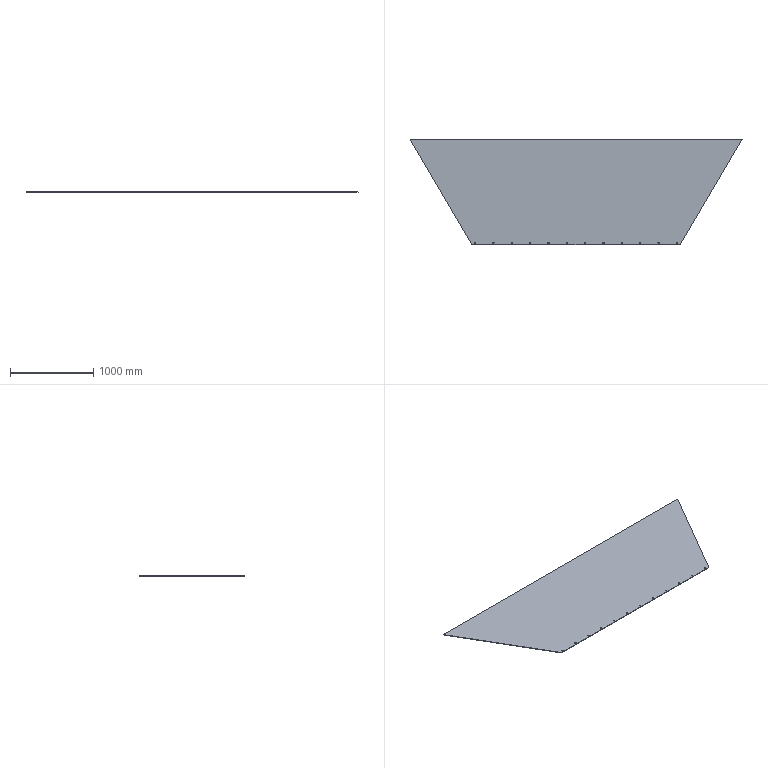Part | SolidWorks | features ICE 3, LPattern 2, FlatPattern 1, SMBaseFlange 1, SheetMetal 1 | 1 solid | 30 faces | box 3983 x 1270 x 6 mm | volume 24689146 mm3 | cylinder 24 | plane 6 | commonest cylinder face diameters 14 x24
STEP:
#1=CARTESIAN_POINT('',(-1203.,-610.,-6.));
#2=VERTEX_POINT('',#1);
#3=CARTESIAN_POINT('',(-1217.,-610.,-6.));
#4=VERTEX_POINT('',#3);
#5=CARTESIAN_POINT('',(-1210.,-610.,-6.));
#6=DIRECTION('',(0.,0.,-1.));
#7=DIRECTION('',(1.,0.,0.));
#8=AXIS2_PLACEMENT_3D('',#5,#6,#7);
#9=CIRCLE('',#8,7.);
#10=EDGE_CURVE('',#2,#4,#9,.T.);
#11=ORIENTED_EDGE('',*,*,#10,.T.);
#12=CARTESIAN_POINT('',(-1217.,-610.,0.));
#13=VERTEX_POINT('',#12);
#14=CARTESIAN_POINT('',(-1217.,-610.,-6.001));
#15=DIRECTION('',(0.,0.,1.));
#16=VECTOR('',#15,1000.);
#17=LINE('',#14,#16);
#18=EDGE_CURVE('',#4,#13,#17,.T.);
#19=ORIENTED_EDGE('',*,*,#18,.T.);
#20=CARTESIAN_POINT('',(-1203.,-610.,0.));
#21=VERTEX_POINT('',#20);
#22=CARTESIAN_POINT('',(-1210.,-610.,0.));
#23=DIRECTION('',(0.,0.,1.));
#24=DIRECTION('',(1.,0.,0.));
#25=AXIS2_PLACEMENT_3D('',#22,#23,#24);
#26=CIRCLE('',#25,7.);
#27=EDGE_CURVE('',#13,#21,#26,.T.);
#28=ORIENTED_EDGE('',*,*,#27,.T.);
#29=CARTESIAN_POINT('',(-1203.,-610.,-6.001));
#30=DIRECTION('',(0.,0.,1.));
#31=VECTOR('',#30,1000.);
#32=LINE('',#29,#31);
#33=EDGE_CURVE('',#2,#21,#32,.T.);
#34=ORIENTED_EDGE('',*,*,#33,.F.);
#35=EDGE_LOOP('',(#11,#19,#28,#34));
#36=FACE_OUTER_BOUND('',#35,.T.);
#37=CARTESIAN_POINT('',(-1210.,-610.,-6.001));
#38=DIRECTION('',(0.,0.,1.));
#39=DIRECTION('',(1.,0.,0.));
#40=AXIS2_PLACEMENT_3D('',#37,#38,#39);
#41=CYLINDRICAL_SURFACE('',#40,7.);
#42=ADVANCED_FACE('',(#36),#41,.F.);
#43=CARTESIAN_POINT('',(-983.,-610.,-6.));
#44=VERTEX_POINT('',#43);
#45=CARTESIAN_POINT('',(-997.,-610.,-6.));
#46=VERTEX_POINT('',#45);
#47=CARTESIAN_POINT('',(-990.,-610.,-6.));
#48=DIRECTION('',(0.,0.,-1.));
#49=DIRECTION('',(1.,0.,0.));
#50=AXIS2_PLACEMENT_3D('',#47,#48,#49);
#51=CIRCLE('',#50,7.);
#52=EDGE_CURVE('',#44,#46,#51,.T.);
#53=ORIENTED_EDGE('',*,*,#52,.T.);
#54=CARTESIAN_POINT('',(-997.,-610.,0.));
#55=VERTEX_POINT('',#54);
#56=CARTESIAN_POINT('',(-997.,-610.,-6.001));
#57=DIRECTION('',(0.,0.,1.));
#58=VECTOR('',#57,1000.);
#59=LINE('',#56,#58);
#60=EDGE_CURVE('',#46,#55,#59,.T.);
#61=ORIENTED_EDGE('',*,*,#60,.T.);
#62=CARTESIAN_POINT('',(-983.,-610.,0.));
#63=VERTEX_POINT('',#62);
#64=CARTESIAN_POINT('',(-990.,-610.,0.));
#65=DIRECTION('',(0.,0.,1.));
#66=DIRECTION('',(1.,0.,0.));
#67=AXIS2_PLACEMENT_3D('',#64,#65,#66);
#68=CIRCLE('',#67,7.);
#69=EDGE_CURVE('',#55,#63,#68,.T.);
#70=ORIENTED_EDGE('',*,*,#69,.T.);
#71=CARTESIAN_POINT('',(-983.,-610.,-6.001));
#72=DIRECTION('',(0.,0.,1.));
#73=VECTOR('',#72,1000.);
#74=LINE('',#71,#73);
#75=EDGE_CURVE('',#44,#63,#74,.T.);
#76=ORIENTED_EDGE('',*,*,#75,.F.);
#77=EDGE_LOOP('',(#53,#61,#70,#76));
#78=FACE_OUTER_BOUND('',#77,.T.);
#79=CARTESIAN_POINT('',(-990.,-610.,-6.001));
#80=DIRECTION('',(0.,0.,1.));
#81=DIRECTION('',(1.,0.,0.));
#82=AXIS2_PLACEMENT_3D('',#79,#80,#81);
#83=CYLINDRICAL_SURFACE('',#82,7.);
#84=ADVANCED_FACE('',(#78),#83,.F.);
#85=CARTESIAN_POINT('',(-763.,-610.,-6.));
#86=VERTEX_POINT('',#85);
#87=CARTESIAN_POINT('',(-777.,-610.,-6.));
#88=VERTEX_POINT('',#87);
#89=CARTESIAN_POINT('',(-770.,-610.,-6.));
#90=DIRECTION('',(0.,0.,-1.));
#91=DIRECTION('',(1.,0.,0.));
#92=AXIS2_PLACEMENT_3D('',#89,#90,#91);
#93=CIRCLE('',#92,7.);
#94=EDGE_CURVE('',#86,#88,#93,.T.);
#95=ORIENTED_EDGE('',*,*,#94,.T.);
#96=CARTESIAN_POINT('',(-777.,-610.,0.));
#97=VERTEX_POINT('',#96);
#98=CARTESIAN_POINT('',(-777.,-610.,-6.001));
#99=DIRECTION('',(0.,0.,1.));
#100=VECTOR('',#99,1000.);
#101=LINE('',#98,#100);
#102=EDGE_CURVE('',#88,#97,#101,.T.);
#103=ORIENTED_EDGE('',*,*,#102,.T.);
#104=CARTESIAN_POINT('',(-763.,-610.,0.));
#105=VERTEX_POINT('',#104);
#106=CARTESIAN_POINT('',(-770.,-610.,0.));
#107=DIRECTION('',(0.,0.,1.));
#108=DIRECTION('',(1.,0.,0.));
#109=AXIS2_PLACEMENT_3D('',#106,#107,#108);
#110=CIRCLE('',#109,7.);
#111=EDGE_CURVE('',#97,#105,#110,.T.);
#112=ORIENTED_EDGE('',*,*,#111,.T.);
#113=CARTESIAN_POINT('',(-763.,-610.,-6.001));
#114=DIRECTION('',(0.,0.,1.));
#115=VECTOR('',#114,1000.);
#116=LINE('',#113,#115);
#117=EDGE_CURVE('',#86,#105,#116,.T.);
#118=ORIENTED_EDGE('',*,*,#117,.F.);
#119=EDGE_LOOP('',(#95,#103,#112,#118));
#120=FACE_OUTER_BOUND('',#119,.T.);
#121=CARTESIAN_POINT('',(-770.,-610.,-6.001));
#122=DIRECTION('',(0.,0.,1.));
#123=DIRECTION('',(1.,0.,0.));
#124=AXIS2_PLACEMENT_3D('',#121,#122,#123);
#125=CYLINDRICAL_SURFACE('',#124,7.);
#126=ADVANCED_FACE('',(#120),#125,.F.);
#127=CARTESIAN_POINT('',(-543.,-610.,-6.));
#128=VERTEX_POINT('',#127);
#129=CARTESIAN_POINT('',(-557.,-610.,-6.));
#130=VERTEX_POINT('',#129);
#131=CARTESIAN_POINT('',(-550.,-610.,-6.));
#132=DIRECTION('',(0.,0.,-1.));
#133=DIRECTION('',(1.,0.,0.));
#134=AXIS2_PLACEMENT_3D('',#131,#132,#133);
#135=CIRCLE('',#134,7.);
#136=EDGE_CURVE('',#128,#130,#135,.T.);
#137=ORIENTED_EDGE('',*,*,#136,.T.);
#138=CARTESIAN_POINT('',(-557.,-610.,0.));
#139=VERTEX_POINT('',#138);
#140=CARTESIAN_POINT('',(-557.,-610.,-6.001));
#141=DIRECTION('',(0.,0.,1.));
#142=VECTOR('',#141,1000.);
#143=LINE('',#140,#142);
#144=EDGE_CURVE('',#130,#139,#143,.T.);
#145=ORIENTED_EDGE('',*,*,#144,.T.);
#146=CARTESIAN_POINT('',(-543.,-610.,0.));
#147=VERTEX_POINT('',#146);
#148=CARTESIAN_POINT('',(-550.,-610.,0.));
#149=DIRECTION('',(0.,0.,1.));
#150=DIRECTION('',(1.,0.,0.));
#151=AXIS2_PLACEMENT_3D('',#148,#149,#150);
#152=CIRCLE('',#151,7.);
#153=EDGE_CURVE('',#139,#147,#152,.T.);
#154=ORIENTED_EDGE('',*,*,#153,.T.);
#155=CARTESIAN_POINT('',(-543.,-610.,-6.001));
#156=DIRECTION('',(0.,0.,1.));
#157=VECTOR('',#156,1000.);
#158=LINE('',#155,#157);
#159=EDGE_CURVE('',#128,#147,#158,.T.);
#160=ORIENTED_EDGE('',*,*,#159,.F.);
#161=EDGE_LOOP('',(#137,#145,#154,#160));
#162=FACE_OUTER_BOUND('',#161,.T.);
#163=CARTESIAN_POINT('',(-550.,-610.,-6.001));
#164=DIRECTION('',(0.,0.,1.));
#165=DIRECTION('',(1.,0.,0.));
#166=AXIS2_PLACEMENT_3D('',#163,#164,#165);
#167=CYLINDRICAL_SURFACE('',#166,7.);
#168=ADVANCED_FACE('',(#162),#167,.F.);
#169=CARTESIAN_POINT('',(-323.,-610.,-6.));
#170=VERTEX_POINT('',#169);
#171=CARTESIAN_POINT('',(-337.,-610.,-6.));
#172=VERTEX_POINT('',#171);
#173=CARTESIAN_POINT('',(-330.,-610.,-6.));
#174=DIRECTION('',(0.,0.,-1.));
#175=DIRECTION('',(1.,0.,0.));
#176=AXIS2_PLACEMENT_3D('',#173,#174,#175);
#177=CIRCLE('',#176,7.);
#178=EDGE_CURVE('',#170,#172,#177,.T.);
#179=ORIENTED_EDGE('',*,*,#178,.T.);
#180=CARTESIAN_POINT('',(-337.,-610.,0.));
#181=VERTEX_POINT('',#180);
#182=CARTESIAN_POINT('',(-337.,-610.,-6.001));
#183=DIRECTION('',(0.,0.,1.));
#184=VECTOR('',#183,1000.);
#185=LINE('',#182,#184);
#186=EDGE_CURVE('',#172,#181,#185,.T.);
#187=ORIENTED_EDGE('',*,*,#186,.T.);
#188=CARTESIAN_POINT('',(-323.,-610.,0.));
#189=VERTEX_POINT('',#188);
#190=CARTESIAN_POINT('',(-330.,-610.,0.));
#191=DIRECTION('',(0.,0.,1.));
#192=DIRECTION('',(1.,0.,0.));
#193=AXIS2_PLACEMENT_3D('',#190,#191,#192);
#194=CIRCLE('',#193,7.);
#195=EDGE_CURVE('',#181,#189,#194,.T.);
#196=ORIENTED_EDGE('',*,*,#195,.T.);
#197=CARTESIAN_POINT('',(-323.,-610.,-6.001));
#198=DIRECTION('',(0.,0.,1.));
#199=VECTOR('',#198,1000.);
#200=LINE('',#197,#199);
#201=EDGE_CURVE('',#170,#189,#200,.T.);
#202=ORIENTED_EDGE('',*,*,#201,.F.);
#203=EDGE_LOOP('',(#179,#187,#196,#202));
#204=FACE_OUTER_BOUND('',#203,.T.);
#205=CARTESIAN_POINT('',(-330.,-610.,-6.001));
#206=DIRECTION('',(0.,0.,1.));
#207=DIRECTION('',(1.,0.,0.));
#208=AXIS2_PLACEMENT_3D('',#205,#206,#207);
#209=CYLINDRICAL_SURFACE('',#208,7.);
#210=ADVANCED_FACE('',(#204),#209,.F.);
#211=CARTESIAN_POINT('',(1203.,-610.,-6.));
#212=VERTEX_POINT('',#211);
#213=CARTESIAN_POINT('',(1217.,-610.,-6.));
#214=VERTEX_POINT('',#213);
#215=CARTESIAN_POINT('',(1210.,-610.,-6.));
#216=DIRECTION('',(0.,0.,1.));
#217=DIRECTION('',(1.,0.,0.));
#218=AXIS2_PLACEMENT_3D('',#215,#216,#217);
#219=CIRCLE('',#218,7.);
#220=EDGE_CURVE('',#212,#214,#219,.T.);
#221=ORIENTED_EDGE('',*,*,#220,.F.);
#222=CARTESIAN_POINT('',(1203.,-610.,0.));
#223=VERTEX_POINT('',#222);
#224=CARTESIAN_POINT('',(1203.,-610.,-10.));
#225=DIRECTION('',(0.,0.,1.));
#226=VECTOR('',#225,1000.);
#227=LINE('',#224,#226);
#228=EDGE_CURVE('',#212,#223,#227,.T.);
#229=ORIENTED_EDGE('',*,*,#228,.T.);
#230=CARTESIAN_POINT('',(1217.,-610.,0.));
#231=VERTEX_POINT('',#230);
#232=CARTESIAN_POINT('',(1210.,-610.,0.));
#233=DIRECTION('',(0.,0.,1.));
#234=DIRECTION('',(1.,0.,0.));
#235=AXIS2_PLACEMENT_3D('',#232,#233,#234);
#236=CIRCLE('',#235,7.);
#237=EDGE_CURVE('',#223,#231,#236,.T.);
#238=ORIENTED_EDGE('',*,*,#237,.T.);
#239=CARTESIAN_POINT('',(1217.,-610.,-10.));
#240=DIRECTION('',(0.,0.,1.));
#241=VECTOR('',#240,1000.);
#242=LINE('',#239,#241);
#243=EDGE_CURVE('',#214,#231,#242,.T.);
#244=ORIENTED_EDGE('',*,*,#243,.F.);
#245=EDGE_LOOP('',(#221,#229,#238,#244));
#246=FACE_OUTER_BOUND('',#245,.T.);
#247=CARTESIAN_POINT('',(1210.,-610.,-10.));
#248=DIRECTION('',(0.,0.,1.));
#249=DIRECTION('',(1.,0.,0.));
#250=AXIS2_PLACEMENT_3D('',#247,#248,#249);
#251=CYLINDRICAL_SURFACE('',#250,7.);
#252=ADVANCED_FACE('',(#246),#251,.F.);
#253=CARTESIAN_POINT('',(983.,-610.,-6.));
#254=VERTEX_POINT('',#253);
#255=CARTESIAN_POINT('',(997.,-610.,-6.));
#256=VERTEX_POINT('',#255);
#257=CARTESIAN_POINT('',(990.,-610.,-6.));
#258=DIRECTION('',(0.,0.,1.));
#259=DIRECTION('',(1.,0.,0.));
#260=AXIS2_PLACEMENT_3D('',#257,#258,#259);
#261=CIRCLE('',#260,7.);
#262=EDGE_CURVE('',#254,#256,#261,.T.);
#263=ORIENTED_EDGE('',*,*,#262,.F.);
#264=CARTESIAN_POINT('',(983.,-610.,0.));
#265=VERTEX_POINT('',#264);
#266=CARTESIAN_POINT('',(983.,-610.,-10.));
#267=DIRECTION('',(0.,0.,1.));
#268=VECTOR('',#267,1000.);
#269=LINE('',#266,#268);
#270=EDGE_CURVE('',#254,#265,#269,.T.);
#271=ORIENTED_EDGE('',*,*,#270,.T.);
#272=CARTESIAN_POINT('',(997.,-610.,0.));
#273=VERTEX_POINT('',#272);
#274=CARTESIAN_POINT('',(990.,-610.,0.));
#275=DIRECTION('',(0.,0.,1.));
#276=DIRECTION('',(1.,0.,0.));
#277=AXIS2_PLACEMENT_3D('',#274,#275,#276);
#278=CIRCLE('',#277,7.);
#279=EDGE_CURVE('',#265,#273,#278,.T.);
#280=ORIENTED_EDGE('',*,*,#279,.T.);
#281=CARTESIAN_POINT('',(997.,-610.,-10.));
#282=DIRECTION('',(0.,0.,1.));
#283=VECTOR('',#282,1000.);
#284=LINE('',#281,#283);
#285=EDGE_CURVE('',#256,#273,#284,.T.);
#286=ORIENTED_EDGE('',*,*,#285,.F.);
#287=EDGE_LOOP('',(#263,#271,#280,#286));
#288=FACE_OUTER_BOUND('',#287,.T.);
#289=CARTESIAN_POINT('',(990.,-610.,-10.));
#290=DIRECTION('',(0.,0.,1.));
#291=DIRECTION('',(1.,0.,0.));
#292=AXIS2_PLACEMENT_3D('',#289,#290,#291);
#293=CYLINDRICAL_SURFACE('',#292,7.);
#294=ADVANCED_FACE('',(#288),#293,.F.);
#295=CARTESIAN_POINT('',(763.,-610.,-6.));
#296=VERTEX_POINT('',#295);
#297=CARTESIAN_POINT('',(777.,-610.,-6.));
#298=VERTEX_POINT('',#297);
#299=CARTESIAN_POINT('',(770.,-610.,-6.));
#300=DIRECTION('',(0.,0.,1.));
#301=DIRECTION('',(1.,0.,0.));
#302=AXIS2_PLACEMENT_3D('',#299,#300,#301);
#303=CIRCLE('',#302,7.);
#304=EDGE_CURVE('',#296,#298,#303,.T.);
#305=ORIENTED_EDGE('',*,*,#304,.F.);
#306=CARTESIAN_POINT('',(763.,-610.,0.));
#307=VERTEX_POINT('',#306);
#308=CARTESIAN_POINT('',(763.,-610.,-10.));
#309=DIRECTION('',(0.,0.,1.));
#310=VECTOR('',#309,1000.);
#311=LINE('',#308,#310);
#312=EDGE_CURVE('',#296,#307,#311,.T.);
#313=ORIENTED_EDGE('',*,*,#312,.T.);
#314=CARTESIAN_POINT('',(777.,-610.,0.));
#315=VERTEX_POINT('',#314);
#316=CARTESIAN_POINT('',(770.,-610.,0.));
#317=DIRECTION('',(0.,0.,1.));
#318=DIRECTION('',(1.,0.,0.));
#319=AXIS2_PLACEMENT_3D('',#316,#317,#318);
#320=CIRCLE('',#319,7.);
#321=EDGE_CURVE('',#307,#315,#320,.T.);
#322=ORIENTED_EDGE('',*,*,#321,.T.);
#323=CARTESIAN_POINT('',(777.,-610.,-10.));
#324=DIRECTION('',(0.,0.,1.));
#325=VECTOR('',#324,1000.);
#326=LINE('',#323,#325);
#327=EDGE_CURVE('',#298,#315,#326,.T.);
#328=ORIENTED_EDGE('',*,*,#327,.F.);
#329=EDGE_LOOP('',(#305,#313,#322,#328));
#330=FACE_OUTER_BOUND('',#329,.T.);
#331=CARTESIAN_POINT('',(770.,-610.,-10.));
#332=DIRECTION('',(0.,0.,1.));
#333=DIRECTION('',(1.,0.,0.));
#334=AXIS2_PLACEMENT_3D('',#331,#332,#333);
#335=CYLINDRICAL_SURFACE('',#334,7.);
#336=ADVANCED_FACE('',(#330),#335,.F.);
#337=CARTESIAN_POINT('',(543.,-610.,-6.));
#338=VERTEX_POINT('',#337);
#339=CARTESIAN_POINT('',(557.,-610.,-6.));
#340=VERTEX_POINT('',#339);
#341=CARTESIAN_POINT('',(550.,-610.,-6.));
#342=DIRECTION('',(0.,0.,1.));
#343=DIRECTION('',(1.,0.,0.));
#344=AXIS2_PLACEMENT_3D('',#341,#342,#343);
#345=CIRCLE('',#344,7.);
#346=EDGE_CURVE('',#338,#340,#345,.T.);
#347=ORIENTED_EDGE('',*,*,#346,.F.);
#348=CARTESIAN_POINT('',(543.,-610.,0.));
#349=VERTEX_POINT('',#348);
#350=CARTESIAN_POINT('',(543.,-610.,-10.));
#351=DIRECTION('',(0.,0.,1.));
#352=VECTOR('',#351,1000.);
#353=LINE('',#350,#352);
#354=EDGE_CURVE('',#338,#349,#353,.T.);
#355=ORIENTED_EDGE('',*,*,#354,.T.);
#356=CARTESIAN_POINT('',(557.,-610.,0.));
#357=VERTEX_POINT('',#356);
#358=CARTESIAN_POINT('',(550.,-610.,0.));
#359=DIRECTION('',(0.,0.,1.));
#360=DIRECTION('',(1.,0.,0.));
#361=AXIS2_PLACEMENT_3D('',#358,#359,#360);
#362=CIRCLE('',#361,7.);
#363=EDGE_CURVE('',#349,#357,#362,.T.);
#364=ORIENTED_EDGE('',*,*,#363,.T.);
#365=CARTESIAN_POINT('',(557.,-610.,-10.));
#366=DIRECTION('',(0.,0.,1.));
#367=VECTOR('',#366,1000.);
#368=LINE('',#365,#367);
#369=EDGE_CURVE('',#340,#357,#368,.T.);
#370=ORIENTED_EDGE('',*,*,#369,.F.);
#371=EDGE_LOOP('',(#347,#355,#364,#370));
#372=FACE_OUTER_BOUND('',#371,.T.);
#373=CARTESIAN_POINT('',(550.,-610.,-10.));
#374=DIRECTION('',(0.,0.,1.));
#375=DIRECTION('',(1.,0.,0.));
#376=AXIS2_PLACEMENT_3D('',#373,#374,#375);
#377=CYLINDRICAL_SURFACE('',#376,7.);
#378=ADVANCED_FACE('',(#372),#377,.F.);
#379=CARTESIAN_POINT('',(323.,-610.,-6.));
#380=VERTEX_POINT('',#379);
#381=CARTESIAN_POINT('',(337.,-610.,-6.));
#382=VERTEX_POINT('',#381);
#383=CARTESIAN_POINT('',(330.,-610.,-6.));
#384=DIRECTION('',(0.,0.,1.));
#385=DIRECTION('',(1.,0.,0.));
#386=AXIS2_PLACEMENT_3D('',#383,#384,#385);
#387=CIRCLE('',#386,7.);
#388=EDGE_CURVE('',#380,#382,#387,.T.);
#389=ORIENTED_EDGE('',*,*,#388,.F.);
#390=CARTESIAN_POINT('',(323.,-610.,0.));
#391=VERTEX_POINT('',#390);
#392=CARTESIAN_POINT('',(323.,-610.,-10.));
#393=DIRECTION('',(0.,0.,1.));
#394=VECTOR('',#393,1000.);
#395=LINE('',#392,#394);
#396=EDGE_CURVE('',#380,#391,#395,.T.);
#397=ORIENTED_EDGE('',*,*,#396,.T.);
#398=CARTESIAN_POINT('',(337.,-610.,0.));
#399=VERTEX_POINT('',#398);
#400=CARTESIAN_POINT('',(330.,-610.,0.));
#401=DIRECTION('',(0.,0.,1.));
#402=DIRECTION('',(1.,0.,0.));
#403=AXIS2_PLACEMENT_3D('',#400,#401,#402);
#404=CIRCLE('',#403,7.);
#405=EDGE_CURVE('',#391,#399,#404,.T.);
#406=ORIENTED_EDGE('',*,*,#405,.T.);
#407=CARTESIAN_POINT('',(337.,-610.,-10.));
#408=DIRECTION('',(0.,0.,1.));
#409=VECTOR('',#408,1000.);
#410=LINE('',#407,#409);
#411=EDGE_CURVE('',#382,#399,#410,.T.);
#412=ORIENTED_EDGE('',*,*,#411,.F.);
#413=EDGE_LOOP('',(#389,#397,#406,#412));
#414=FACE_OUTER_BOUND('',#413,.T.);
#415=CARTESIAN_POINT('',(330.,-610.,-10.));
#416=DIRECTION('',(0.,0.,1.));
#417=DIRECTION('',(1.,0.,0.));
#418=AXIS2_PLACEMENT_3D('',#415,#416,#417);
#419=CYLINDRICAL_SURFACE('',#418,7.);
#420=ADVANCED_FACE('',(#414),#419,.F.);
#421=CARTESIAN_POINT('',(-103.,-610.,-6.));
#422=VERTEX_POINT('',#421);
#423=CARTESIAN_POINT('',(-117.,-610.,-6.));
#424=VERTEX_POINT('',#423);
#425=CARTESIAN_POINT('',(-110.,-610.,-6.));
#426=DIRECTION('',(0.,0.,-1.));
#427=DIRECTION('',(1.,0.,0.));
#428=AXIS2_PLACEMENT_3D('',#425,#426,#427);
#429=CIRCLE('',#428,7.);
#430=EDGE_CURVE('',#422,#424,#429,.T.);
#431=ORIENTED_EDGE('',*,*,#430,.T.);
#432=CARTESIAN_POINT('',(-117.,-610.,0.));
#433=VERTEX_POINT('',#432);
#434=CARTESIAN_POINT('',(-117.,-610.,-6.001));
#435=DIRECTION('',(0.,0.,1.));
#436=VECTOR('',#435,1000.);
#437=LINE('',#434,#436);
#438=EDGE_CURVE('',#424,#433,#437,.T.);
#439=ORIENTED_EDGE('',*,*,#438,.T.);
#440=CARTESIAN_POINT('',(-103.,-610.,0.));
#441=VERTEX_POINT('',#440);
#442=CARTESIAN_POINT('',(-110.,-610.,0.));
#443=DIRECTION('',(0.,0.,1.));
#444=DIRECTION('',(1.,0.,0.));
#445=AXIS2_PLACEMENT_3D('',#442,#443,#444);
#446=CIRCLE('',#445,7.);
#447=EDGE_CURVE('',#433,#441,#446,.T.);
#448=ORIENTED_EDGE('',*,*,#447,.T.);
#449=CARTESIAN_POINT('',(-103.,-610.,-6.001));
#450=DIRECTION('',(0.,0.,1.));
#451=VECTOR('',#450,1000.);
#452=LINE('',#449,#451);
#453=EDGE_CURVE('',#422,#441,#452,.T.);
#454=ORIENTED_EDGE('',*,*,#453,.F.);
#455=EDGE_LOOP('',(#431,#439,#448,#454));
#456=FACE_OUTER_BOUND('',#455,.T.);
#457=CARTESIAN_POINT('',(-110.,-610.,-6.001));
#458=DIRECTION('',(0.,0.,1.));
#459=DIRECTION('',(1.,0.,0.));
#460=AXIS2_PLACEMENT_3D('',#457,#458,#459);
#461=CYLINDRICAL_SURFACE('',#460,7.);
#462=ADVANCED_FACE('',(#456),#461,.F.);
#463=CARTESIAN_POINT('',(103.,-610.,-6.));
#464=VERTEX_POINT('',#463);
#465=CARTESIAN_POINT('',(117.,-610.,-6.));
#466=VERTEX_POINT('',#465);
#467=CARTESIAN_POINT('',(110.,-610.,-6.));
#468=DIRECTION('',(0.,0.,1.));
#469=DIRECTION('',(1.,0.,0.));
#470=AXIS2_PLACEMENT_3D('',#467,#468,#469);
#471=CIRCLE('',#470,7.);
#472=EDGE_CURVE('',#464,#466,#471,.T.);
#473=ORIENTED_EDGE('',*,*,#472,.F.);
#474=CARTESIAN_POINT('',(103.,-610.,0.));
#475=VERTEX_POINT('',#474);
#476=CARTESIAN_POINT('',(103.,-610.,-10.));
#477=DIRECTION('',(0.,0.,1.));
#478=VECTOR('',#477,1000.);
#479=LINE('',#476,#478);
#480=EDGE_CURVE('',#464,#475,#479,.T.);
#481=ORIENTED_EDGE('',*,*,#480,.T.);
#482=CARTESIAN_POINT('',(117.,-610.,0.));
#483=VERTEX_POINT('',#482);
#484=CARTESIAN_POINT('',(110.,-610.,0.));
#485=DIRECTION('',(0.,0.,1.));
#486=DIRECTION('',(1.,0.,0.));
#487=AXIS2_PLACEMENT_3D('',#484,#485,#486);
#488=CIRCLE('',#487,7.);
#489=EDGE_CURVE('',#475,#483,#488,.T.);
#490=ORIENTED_EDGE('',*,*,#489,.T.);
#491=CARTESIAN_POINT('',(117.,-610.,-10.));
#492=DIRECTION('',(0.,0.,1.));
#493=VECTOR('',#492,1000.);
#494=LINE('',#491,#493);
#495=EDGE_CURVE('',#466,#483,#494,.T.);
#496=ORIENTED_EDGE('',*,*,#495,.F.);
#497=EDGE_LOOP('',(#473,#481,#490,#496));
#498=FACE_OUTER_BOUND('',#497,.T.);
#499=CARTESIAN_POINT('',(110.,-610.,-10.));
#500=DIRECTION('',(0.,0.,1.));
#501=DIRECTION('',(1.,0.,0.));
#502=AXIS2_PLACEMENT_3D('',#499,#500,#501);
#503=CYLINDRICAL_SURFACE('',#502,7.);
#504=ADVANCED_FACE('',(#498),#503,.F.);
#505=CARTESIAN_POINT('',(-1250.,-635.,0.));
#506=VERTEX_POINT('',#505);
#507=CARTESIAN_POINT('',(1250.,-635.,0.));
#508=VERTEX_POINT('',#507);
#509=CARTESIAN_POINT('',(1991.5,-635.,0.));
#510=DIRECTION('',(1.,0.,0.));
#511=VECTOR('',#510,1000.);
#512=LINE('',#509,#511);
#513=EDGE_CURVE('',#506,#508,#512,.T.);
#514=ORIENTED_EDGE('',*,*,#513,.F.);
#515=CARTESIAN_POINT('',(-1250.,-635.,-6.));
#516=VERTEX_POINT('',#515);
#517=CARTESIAN_POINT('',(-1250.,-635.,-6.));
#518=DIRECTION('',(0.,0.,1.));
#519=VECTOR('',#518,1000.);
#520=LINE('',#517,#519);
#521=EDGE_CURVE('',#516,#506,#520,.T.);
#522=ORIENTED_EDGE('',*,*,#521,.F.);
#523=CARTESIAN_POINT('',(1250.,-635.,-6.));
#524=VERTEX_POINT('',#523);
#525=CARTESIAN_POINT('',(1991.5,-635.,-6.));
#526=DIRECTION('',(1.,0.,0.));
#527=VECTOR('',#526,1000.);
#528=LINE('',#525,#527);
#529=EDGE_CURVE('',#516,#524,#528,.T.);
#530=ORIENTED_EDGE('',*,*,#529,.T.);
#531=CARTESIAN_POINT('',(1250.,-635.,-6.));
#532=DIRECTION('',(0.,0.,1.));
#533=VECTOR('',#532,1000.);
#534=LINE('',#531,#533);
#535=EDGE_CURVE('',#524,#508,#534,.T.);
#536=ORIENTED_EDGE('',*,*,#535,.T.);
#537=EDGE_LOOP('',(#514,#522,#530,#536));
#538=FACE_OUTER_BOUND('',#537,.T.);
#539=CARTESIAN_POINT('',(1991.5,-635.,-6.));
#540=DIRECTION('',(0.,-1.,0.));
#541=DIRECTION('',(1.,0.,0.));
#542=AXIS2_PLACEMENT_3D('',#539,#540,#541);
#543=PLANE('',#542);
#544=ADVANCED_FACE('',(#538),#543,.T.);
#545=ORIENTED_EDGE('',*,*,#178,.F.);
#546=CARTESIAN_POINT('',(-330.,-610.,-6.));
#547=DIRECTION('',(0.,0.,-1.));
#548=DIRECTION('',(1.,0.,0.));
#549=AXIS2_PLACEMENT_3D('',#546,#547,#548);
#550=CIRCLE('',#549,7.);
#551=EDGE_CURVE('',#172,#170,#550,.T.);
#552=ORIENTED_EDGE('',*,*,#551,.F.);
#553=EDGE_LOOP('',(#545,#552));
#554=FACE_BOUND('',#553,.T.);
#555=CARTESIAN_POINT('',(330.,-610.,-6.));
#556=DIRECTION('',(0.,0.,1.));
#557=DIRECTION('',(1.,0.,0.));
#558=AXIS2_PLACEMENT_3D('',#555,#556,#557);
#559=CIRCLE('',#558,7.);
#560=EDGE_CURVE('',#382,#380,#559,.T.);
#561=ORIENTED_EDGE('',*,*,#560,.T.);
#562=ORIENTED_EDGE('',*,*,#388,.T.);
#563=EDGE_LOOP('',(#561,#562));
#564=FACE_BOUND('',#563,.T.);
#565=ORIENTED_EDGE('',*,*,#430,.F.);
#566=CARTESIAN_POINT('',(-110.,-610.,-6.));
#567=DIRECTION('',(0.,0.,-1.));
#568=DIRECTION('',(1.,0.,0.));
#569=AXIS2_PLACEMENT_3D('',#566,#567,#568);
#570=CIRCLE('',#569,7.);
#571=EDGE_CURVE('',#424,#422,#570,.T.);
#572=ORIENTED_EDGE('',*,*,#571,.F.);
#573=EDGE_LOOP('',(#565,#572));
#574=FACE_BOUND('',#573,.T.);
#575=CARTESIAN_POINT('',(110.,-610.,-6.));
#576=DIRECTION('',(0.,0.,1.));
#577=DIRECTION('',(1.,0.,0.));
#578=AXIS2_PLACEMENT_3D('',#575,#576,#577);
#579=CIRCLE('',#578,7.);
#580=EDGE_CURVE('',#466,#464,#579,.T.);
#581=ORIENTED_EDGE('',*,*,#580,.T.);
#582=ORIENTED_EDGE('',*,*,#472,.T.);
#583=EDGE_LOOP('',(#581,#582));
#584=FACE_BOUND('',#583,.T.);
#585=CARTESIAN_POINT('',(-1991.5,635.,-6.));
#586=VERTEX_POINT('',#585);
#587=CARTESIAN_POINT('',(-1991.5,635.,-6.));
#588=DIRECTION('',(0.5042,-0.8636,0.));
#589=VECTOR('',#588,1000.);
#590=LINE('',#587,#589);
#591=EDGE_CURVE('',#586,#516,#590,.T.);
#592=ORIENTED_EDGE('',*,*,#591,.F.);
#593=CARTESIAN_POINT('',(1991.5,635.,-6.));
#594=VERTEX_POINT('',#593);
#595=CARTESIAN_POINT('',(1991.5,635.,-6.));
#596=DIRECTION('',(-1.,0.,0.));
#597=VECTOR('',#596,1000.);
#598=LINE('',#595,#597);
#599=EDGE_CURVE('',#594,#586,#598,.T.);
#600=ORIENTED_EDGE('',*,*,#599,.F.);
#601=CARTESIAN_POINT('',(1991.5,635.,-6.));
#602=DIRECTION('',(0.5042,0.8636,0.));
#603=VECTOR('',#602,1000.);
#604=LINE('',#601,#603);
#605=EDGE_CURVE('',#524,#594,#604,.T.);
#606=ORIENTED_EDGE('',*,*,#605,.F.);
#607=ORIENTED_EDGE('',*,*,#529,.F.);
#608=EDGE_LOOP('',(#592,#600,#606,#607));
#609=FACE_OUTER_BOUND('',#608,.T.);
#610=CARTESIAN_POINT('',(550.,-610.,-6.));
#611=DIRECTION('',(0.,0.,1.));
#612=DIRECTION('',(1.,0.,0.));
#613=AXIS2_PLACEMENT_3D('',#610,#611,#612);
#614=CIRCLE('',#613,7.);
#615=EDGE_CURVE('',#340,#338,#614,.T.);
#616=ORIENTED_EDGE('',*,*,#615,.T.);
#617=ORIENTED_EDGE('',*,*,#346,.T.);
#618=EDGE_LOOP('',(#616,#617));
#619=FACE_BOUND('',#618,.T.);
#620=CARTESIAN_POINT('',(770.,-610.,-6.));
#621=DIRECTION('',(0.,0.,1.));
#622=DIRECTION('',(1.,0.,0.));
#623=AXIS2_PLACEMENT_3D('',#620,#621,#622);
#624=CIRCLE('',#623,7.);
#625=EDGE_CURVE('',#298,#296,#624,.T.);
#626=ORIENTED_EDGE('',*,*,#625,.T.);
#627=ORIENTED_EDGE('',*,*,#304,.T.);
#628=EDGE_LOOP('',(#626,#627));
#629=FACE_BOUND('',#628,.T.);
#630=CARTESIAN_POINT('',(990.,-610.,-6.));
#631=DIRECTION('',(0.,0.,1.));
#632=DIRECTION('',(1.,0.,0.));
#633=AXIS2_PLACEMENT_3D('',#630,#631,#632);
#634=CIRCLE('',#633,7.);
#635=EDGE_CURVE('',#256,#254,#634,.T.);
#636=ORIENTED_EDGE('',*,*,#635,.T.);
#637=ORIENTED_EDGE('',*,*,#262,.T.);
#638=EDGE_LOOP('',(#636,#637));
#639=FACE_BOUND('',#638,.T.);
#640=CARTESIAN_POINT('',(1210.,-610.,-6.));
#641=DIRECTION('',(0.,0.,1.));
#642=DIRECTION('',(1.,0.,0.));
#643=AXIS2_PLACEMENT_3D('',#640,#641,#642);
#644=CIRCLE('',#643,7.);
#645=EDGE_CURVE('',#214,#212,#644,.T.);
#646=ORIENTED_EDGE('',*,*,#645,.T.);
#647=ORIENTED_EDGE('',*,*,#220,.T.);
#648=EDGE_LOOP('',(#646,#647));
#649=FACE_BOUND('',#648,.T.);
#650=ORIENTED_EDGE('',*,*,#136,.F.);
#651=CARTESIAN_POINT('',(-550.,-610.,-6.));
#652=DIRECTION('',(0.,0.,-1.));
#653=DIRECTION('',(1.,0.,0.));
#654=AXIS2_PLACEMENT_3D('',#651,#652,#653);
#655=CIRCLE('',#654,7.);
#656=EDGE_CURVE('',#130,#128,#655,.T.);
#657=ORIENTED_EDGE('',*,*,#656,.F.);
#658=EDGE_LOOP('',(#650,#657));
#659=FACE_BOUND('',#658,.T.);
#660=ORIENTED_EDGE('',*,*,#94,.F.);
#661=CARTESIAN_POINT('',(-770.,-610.,-6.));
#662=DIRECTION('',(0.,0.,-1.));
#663=DIRECTION('',(1.,0.,0.));
#664=AXIS2_PLACEMENT_3D('',#661,#662,#663);
#665=CIRCLE('',#664,7.);
#666=EDGE_CURVE('',#88,#86,#665,.T.);
#667=ORIENTED_EDGE('',*,*,#666,.F.);
#668=EDGE_LOOP('',(#660,#667));
#669=FACE_BOUND('',#668,.T.);
#670=ORIENTED_EDGE('',*,*,#52,.F.);
#671=CARTESIAN_POINT('',(-990.,-610.,-6.));
#672=DIRECTION('',(0.,0.,-1.));
#673=DIRECTION('',(1.,0.,0.));
#674=AXIS2_PLACEMENT_3D('',#671,#672,#673);
#675=CIRCLE('',#674,7.);
#676=EDGE_CURVE('',#46,#44,#675,.T.);
#677=ORIENTED_EDGE('',*,*,#676,.F.);
#678=EDGE_LOOP('',(#670,#677));
#679=FACE_BOUND('',#678,.T.);
#680=ORIENTED_EDGE('',*,*,#10,.F.);
#681=CARTESIAN_POINT('',(-1210.,-610.,-6.));
#682=DIRECTION('',(0.,0.,-1.));
#683=DIRECTION('',(1.,0.,0.));
#684=AXIS2_PLACEMENT_3D('',#681,#682,#683);
#685=CIRCLE('',#684,7.);
#686=EDGE_CURVE('',#4,#2,#685,.T.);
#687=ORIENTED_EDGE('',*,*,#686,.F.);
#688=EDGE_LOOP('',(#680,#687));
#689=FACE_BOUND('',#688,.T.);
#690=CARTESIAN_POINT('',(0.,0.,-6.));
#691=DIRECTION('',(0.,0.,1.));
#692=DIRECTION('',(1.,0.,0.));
#693=AXIS2_PLACEMENT_3D('',#690,#691,#692);
#694=PLANE('',#693);
#695=ADVANCED_FACE('',(#554,#564,#574,#584,#609,#619,#629,#639,#649,#659,#669,#679,#689),#694,.F.);
#696=CARTESIAN_POINT('',(-330.,-610.,0.));
#697=DIRECTION('',(0.,0.,1.));
#698=DIRECTION('',(1.,0.,0.));
#699=AXIS2_PLACEMENT_3D('',#696,#697,#698);
#700=CIRCLE('',#699,7.);
#701=EDGE_CURVE('',#189,#181,#700,.T.);
#702=ORIENTED_EDGE('',*,*,#701,.F.);
#703=ORIENTED_EDGE('',*,*,#195,.F.);
#704=EDGE_LOOP('',(#702,#703));
#705=FACE_BOUND('',#704,.T.);
#706=CARTESIAN_POINT('',(330.,-610.,0.));
#707=DIRECTION('',(0.,0.,1.));
#708=DIRECTION('',(1.,0.,0.));
#709=AXIS2_PLACEMENT_3D('',#706,#707,#708);
#710=CIRCLE('',#709,7.);
#711=EDGE_CURVE('',#399,#391,#710,.T.);
#712=ORIENTED_EDGE('',*,*,#711,.F.);
#713=ORIENTED_EDGE('',*,*,#405,.F.);
#714=EDGE_LOOP('',(#712,#713));
#715=FACE_BOUND('',#714,.T.);
#716=CARTESIAN_POINT('',(-110.,-610.,0.));
#717=DIRECTION('',(0.,0.,1.));
#718=DIRECTION('',(1.,0.,0.));
#719=AXIS2_PLACEMENT_3D('',#716,#717,#718);
#720=CIRCLE('',#719,7.);
#721=EDGE_CURVE('',#441,#433,#720,.T.);
#722=ORIENTED_EDGE('',*,*,#721,.F.);
#723=ORIENTED_EDGE('',*,*,#447,.F.);
#724=EDGE_LOOP('',(#722,#723));
#725=FACE_BOUND('',#724,.T.);
#726=CARTESIAN_POINT('',(110.,-610.,0.));
#727=DIRECTION('',(0.,0.,1.));
#728=DIRECTION('',(1.,0.,0.));
#729=AXIS2_PLACEMENT_3D('',#726,#727,#728);
#730=CIRCLE('',#729,7.);
#731=EDGE_CURVE('',#483,#475,#730,.T.);
#732=ORIENTED_EDGE('',*,*,#731,.F.);
#733=ORIENTED_EDGE('',*,*,#489,.F.);
#734=EDGE_LOOP('',(#732,#733));
#735=FACE_BOUND('',#734,.T.);
#736=CARTESIAN_POINT('',(1991.5,635.,0.));
#737=VERTEX_POINT('',#736);
#738=CARTESIAN_POINT('',(-1991.5,635.,0.));
#739=VERTEX_POINT('',#738);
#740=CARTESIAN_POINT('',(1991.5,635.,0.));
#741=DIRECTION('',(-1.,0.,0.));
#742=VECTOR('',#741,1000.);
#743=LINE('',#740,#742);
#744=EDGE_CURVE('',#737,#739,#743,.T.);
#745=ORIENTED_EDGE('',*,*,#744,.T.);
#746=CARTESIAN_POINT('',(-1991.5,635.,0.));
#747=DIRECTION('',(0.5042,-0.8636,0.));
#748=VECTOR('',#747,1000.);
#749=LINE('',#746,#748);
#750=EDGE_CURVE('',#739,#506,#749,.T.);
#751=ORIENTED_EDGE('',*,*,#750,.T.);
#752=ORIENTED_EDGE('',*,*,#513,.T.);
#753=CARTESIAN_POINT('',(1991.5,635.,0.));
#754=DIRECTION('',(0.5042,0.8636,0.));
#755=VECTOR('',#754,1000.);
#756=LINE('',#753,#755);
#757=EDGE_CURVE('',#508,#737,#756,.T.);
#758=ORIENTED_EDGE('',*,*,#757,.T.);
#759=EDGE_LOOP('',(#745,#751,#752,#758));
#760=FACE_OUTER_BOUND('',#759,.T.);
#761=CARTESIAN_POINT('',(550.,-610.,0.));
#762=DIRECTION('',(0.,0.,1.));
#763=DIRECTION('',(1.,0.,0.));
#764=AXIS2_PLACEMENT_3D('',#761,#762,#763);
#765=CIRCLE('',#764,7.);
#766=EDGE_CURVE('',#357,#349,#765,.T.);
#767=ORIENTED_EDGE('',*,*,#766,.F.);
#768=ORIENTED_EDGE('',*,*,#363,.F.);
#769=EDGE_LOOP('',(#767,#768));
#770=FACE_BOUND('',#769,.T.);
#771=CARTESIAN_POINT('',(770.,-610.,0.));
#772=DIRECTION('',(0.,0.,1.));
#773=DIRECTION('',(1.,0.,0.));
#774=AXIS2_PLACEMENT_3D('',#771,#772,#773);
#775=CIRCLE('',#774,7.);
#776=EDGE_CURVE('',#315,#307,#775,.T.);
#777=ORIENTED_EDGE('',*,*,#776,.F.);
#778=ORIENTED_EDGE('',*,*,#321,.F.);
#779=EDGE_LOOP('',(#777,#778));
#780=FACE_BOUND('',#779,.T.);
#781=CARTESIAN_POINT('',(990.,-610.,0.));
#782=DIRECTION('',(0.,0.,1.));
#783=DIRECTION('',(1.,0.,0.));
#784=AXIS2_PLACEMENT_3D('',#781,#782,#783);
#785=CIRCLE('',#784,7.);
#786=EDGE_CURVE('',#273,#265,#785,.T.);
#787=ORIENTED_EDGE('',*,*,#786,.F.);
#788=ORIENTED_EDGE('',*,*,#279,.F.);
#789=EDGE_LOOP('',(#787,#788));
#790=FACE_BOUND('',#789,.T.);
#791=CARTESIAN_POINT('',(1210.,-610.,0.));
#792=DIRECTION('',(0.,0.,1.));
#793=DIRECTION('',(1.,0.,0.));
#794=AXIS2_PLACEMENT_3D('',#791,#792,#793);
#795=CIRCLE('',#794,7.);
#796=EDGE_CURVE('',#231,#223,#795,.T.);
#797=ORIENTED_EDGE('',*,*,#796,.F.);
#798=ORIENTED_EDGE('',*,*,#237,.F.);
#799=EDGE_LOOP('',(#797,#798));
#800=FACE_BOUND('',#799,.T.);
#801=CARTESIAN_POINT('',(-550.,-610.,0.));
#802=DIRECTION('',(0.,0.,1.));
#803=DIRECTION('',(1.,0.,0.));
#804=AXIS2_PLACEMENT_3D('',#801,#802,#803);
#805=CIRCLE('',#804,7.);
#806=EDGE_CURVE('',#147,#139,#805,.T.);
#807=ORIENTED_EDGE('',*,*,#806,.F.);
#808=ORIENTED_EDGE('',*,*,#153,.F.);
#809=EDGE_LOOP('',(#807,#808));
#810=FACE_BOUND('',#809,.T.);
#811=CARTESIAN_POINT('',(-770.,-610.,0.));
#812=DIRECTION('',(0.,0.,1.));
#813=DIRECTION('',(1.,0.,0.));
#814=AXIS2_PLACEMENT_3D('',#811,#812,#813);
#815=CIRCLE('',#814,7.);
#816=EDGE_CURVE('',#105,#97,#815,.T.);
#817=ORIENTED_EDGE('',*,*,#816,.F.);
#818=ORIENTED_EDGE('',*,*,#111,.F.);
#819=EDGE_LOOP('',(#817,#818));
#820=FACE_BOUND('',#819,.T.);
#821=CARTESIAN_POINT('',(-990.,-610.,0.));
#822=DIRECTION('',(0.,0.,1.));
#823=DIRECTION('',(1.,0.,0.));
#824=AXIS2_PLACEMENT_3D('',#821,#822,#823);
#825=CIRCLE('',#824,7.);
#826=EDGE_CURVE('',#63,#55,#825,.T.);
#827=ORIENTED_EDGE('',*,*,#826,.F.);
#828=ORIENTED_EDGE('',*,*,#69,.F.);
#829=EDGE_LOOP('',(#827,#828));
#830=FACE_BOUND('',#829,.T.);
#831=CARTESIAN_POINT('',(-1210.,-610.,0.));
#832=DIRECTION('',(0.,0.,1.));
#833=DIRECTION('',(1.,0.,0.));
#834=AXIS2_PLACEMENT_3D('',#831,#832,#833);
#835=CIRCLE('',#834,7.);
#836=EDGE_CURVE('',#21,#13,#835,.T.);
#837=ORIENTED_EDGE('',*,*,#836,.F.);
#838=ORIENTED_EDGE('',*,*,#27,.F.);
#839=EDGE_LOOP('',(#837,#838));
#840=FACE_BOUND('',#839,.T.);
#841=CARTESIAN_POINT('',(0.,0.,0.));
#842=DIRECTION('',(0.,0.,1.));
#843=DIRECTION('',(1.,0.,0.));
#844=AXIS2_PLACEMENT_3D('',#841,#842,#843);
#845=PLANE('',#844);
#846=ADVANCED_FACE('',(#705,#715,#725,#735,#760,#770,#780,#790,#800,#810,#820,#830,#840),#845,.T.);
#847=ORIENTED_EDGE('',*,*,#744,.F.);
#848=CARTESIAN_POINT('',(1991.5,635.,-6.));
#849=DIRECTION('',(0.,0.,1.));
#850=VECTOR('',#849,1000.);
#851=LINE('',#848,#850);
#852=EDGE_CURVE('',#594,#737,#851,.T.);
#853=ORIENTED_EDGE('',*,*,#852,.F.);
#854=ORIENTED_EDGE('',*,*,#599,.T.);
#855=CARTESIAN_POINT('',(-1991.5,635.,-6.));
#856=DIRECTION('',(0.,0.,1.));
#857=VECTOR('',#856,1000.);
#858=LINE('',#855,#857);
#859=EDGE_CURVE('',#586,#739,#858,.T.);
#860=ORIENTED_EDGE('',*,*,#859,.T.);
#861=EDGE_LOOP('',(#847,#853,#854,#860));
#862=FACE_OUTER_BOUND('',#861,.T.);
#863=CARTESIAN_POINT('',(1991.5,635.,-6.));
#864=DIRECTION('',(0.,1.,0.));
#865=DIRECTION('',(-1.,0.,0.));
#866=AXIS2_PLACEMENT_3D('',#863,#864,#865);
#867=PLANE('',#866);
#868=ADVANCED_FACE('',(#862),#867,.T.);
#869=ORIENTED_EDGE('',*,*,#535,.F.);
#870=ORIENTED_EDGE('',*,*,#605,.T.);
#871=ORIENTED_EDGE('',*,*,#852,.T.);
#872=ORIENTED_EDGE('',*,*,#757,.F.);
#873=EDGE_LOOP('',(#869,#870,#871,#872));
#874=FACE_OUTER_BOUND('',#873,.T.);
#875=CARTESIAN_POINT('',(1991.5,635.,-6.));
#876=DIRECTION('',(0.8636,-0.5042,0.));
#877=DIRECTION('',(0.5042,0.8636,0.));
#878=AXIS2_PLACEMENT_3D('',#875,#876,#877);
#879=PLANE('',#878);
#880=ADVANCED_FACE('',(#874),#879,.T.);
#881=ORIENTED_EDGE('',*,*,#859,.F.);
#882=ORIENTED_EDGE('',*,*,#591,.T.);
#883=ORIENTED_EDGE('',*,*,#521,.T.);
#884=ORIENTED_EDGE('',*,*,#750,.F.);
#885=EDGE_LOOP('',(#881,#882,#883,#884));
#886=FACE_OUTER_BOUND('',#885,.T.);
#887=CARTESIAN_POINT('',(-1991.5,635.,-6.));
#888=DIRECTION('',(-0.8636,-0.5042,0.));
#889=DIRECTION('',(0.5042,-0.8636,0.));
#890=AXIS2_PLACEMENT_3D('',#887,#888,#889);
#891=PLANE('',#890);
#892=ADVANCED_FACE('',(#886),#891,.T.);
#893=ORIENTED_EDGE('',*,*,#480,.F.);
#894=ORIENTED_EDGE('',*,*,#580,.F.);
#895=ORIENTED_EDGE('',*,*,#495,.T.);
#896=ORIENTED_EDGE('',*,*,#731,.T.);
#897=EDGE_LOOP('',(#893,#894,#895,#896));
#898=FACE_OUTER_BOUND('',#897,.T.);
#899=CARTESIAN_POINT('',(110.,-610.,-10.));
#900=DIRECTION('',(0.,0.,1.));
#901=DIRECTION('',(1.,0.,0.));
#902=AXIS2_PLACEMENT_3D('',#899,#900,#901);
#903=CYLINDRICAL_SURFACE('',#902,7.);
#904=ADVANCED_FACE('',(#898),#903,.F.);
#905=ORIENTED_EDGE('',*,*,#438,.F.);
#906=ORIENTED_EDGE('',*,*,#571,.T.);
#907=ORIENTED_EDGE('',*,*,#453,.T.);
#908=ORIENTED_EDGE('',*,*,#721,.T.);
#909=EDGE_LOOP('',(#905,#906,#907,#908));
#910=FACE_OUTER_BOUND('',#909,.T.);
#911=CARTESIAN_POINT('',(-110.,-610.,-6.001));
#912=DIRECTION('',(0.,0.,1.));
#913=DIRECTION('',(1.,0.,0.));
#914=AXIS2_PLACEMENT_3D('',#911,#912,#913);
#915=CYLINDRICAL_SURFACE('',#914,7.);
#916=ADVANCED_FACE('',(#910),#915,.F.);
#917=ORIENTED_EDGE('',*,*,#396,.F.);
#918=ORIENTED_EDGE('',*,*,#560,.F.);
#919=ORIENTED_EDGE('',*,*,#411,.T.);
#920=ORIENTED_EDGE('',*,*,#711,.T.);
#921=EDGE_LOOP('',(#917,#918,#919,#920));
#922=FACE_OUTER_BOUND('',#921,.T.);
#923=CARTESIAN_POINT('',(330.,-610.,-10.));
#924=DIRECTION('',(0.,0.,1.));
#925=DIRECTION('',(1.,0.,0.));
#926=AXIS2_PLACEMENT_3D('',#923,#924,#925);
#927=CYLINDRICAL_SURFACE('',#926,7.);
#928=ADVANCED_FACE('',(#922),#927,.F.);
#929=ORIENTED_EDGE('',*,*,#354,.F.);
#930=ORIENTED_EDGE('',*,*,#615,.F.);
#931=ORIENTED_EDGE('',*,*,#369,.T.);
#932=ORIENTED_EDGE('',*,*,#766,.T.);
#933=EDGE_LOOP('',(#929,#930,#931,#932));
#934=FACE_OUTER_BOUND('',#933,.T.);
#935=CARTESIAN_POINT('',(550.,-610.,-10.));
#936=DIRECTION('',(0.,0.,1.));
#937=DIRECTION('',(1.,0.,0.));
#938=AXIS2_PLACEMENT_3D('',#935,#936,#937);
#939=CYLINDRICAL_SURFACE('',#938,7.);
#940=ADVANCED_FACE('',(#934),#939,.F.);
#941=ORIENTED_EDGE('',*,*,#312,.F.);
#942=ORIENTED_EDGE('',*,*,#625,.F.);
#943=ORIENTED_EDGE('',*,*,#327,.T.);
#944=ORIENTED_EDGE('',*,*,#776,.T.);
#945=EDGE_LOOP('',(#941,#942,#943,#944));
#946=FACE_OUTER_BOUND('',#945,.T.);
#947=CARTESIAN_POINT('',(770.,-610.,-10.));
#948=DIRECTION('',(0.,0.,1.));
#949=DIRECTION('',(1.,0.,0.));
#950=AXIS2_PLACEMENT_3D('',#947,#948,#949);
#951=CYLINDRICAL_SURFACE('',#950,7.);
#952=ADVANCED_FACE('',(#946),#951,.F.);
#953=ORIENTED_EDGE('',*,*,#270,.F.);
#954=ORIENTED_EDGE('',*,*,#635,.F.);
#955=ORIENTED_EDGE('',*,*,#285,.T.);
#956=ORIENTED_EDGE('',*,*,#786,.T.);
#957=EDGE_LOOP('',(#953,#954,#955,#956));
#958=FACE_OUTER_BOUND('',#957,.T.);
#959=CARTESIAN_POINT('',(990.,-610.,-10.));
#960=DIRECTION('',(0.,0.,1.));
#961=DIRECTION('',(1.,0.,0.));
#962=AXIS2_PLACEMENT_3D('',#959,#960,#961);
#963=CYLINDRICAL_SURFACE('',#962,7.);
#964=ADVANCED_FACE('',(#958),#963,.F.);
#965=ORIENTED_EDGE('',*,*,#228,.F.);
#966=ORIENTED_EDGE('',*,*,#645,.F.);
#967=ORIENTED_EDGE('',*,*,#243,.T.);
#968=ORIENTED_EDGE('',*,*,#796,.T.);
#969=EDGE_LOOP('',(#965,#966,#967,#968));
#970=FACE_OUTER_BOUND('',#969,.T.);
#971=CARTESIAN_POINT('',(1210.,-610.,-10.));
#972=DIRECTION('',(0.,0.,1.));
#973=DIRECTION('',(1.,0.,0.));
#974=AXIS2_PLACEMENT_3D('',#971,#972,#973);
#975=CYLINDRICAL_SURFACE('',#974,7.);
#976=ADVANCED_FACE('',(#970),#975,.F.);
#977=ORIENTED_EDGE('',*,*,#186,.F.);
#978=ORIENTED_EDGE('',*,*,#551,.T.);
#979=ORIENTED_EDGE('',*,*,#201,.T.);
#980=ORIENTED_EDGE('',*,*,#701,.T.);
#981=EDGE_LOOP('',(#977,#978,#979,#980));
#982=FACE_OUTER_BOUND('',#981,.T.);
#983=CARTESIAN_POINT('',(-330.,-610.,-6.001));
#984=DIRECTION('',(0.,0.,1.));
#985=DIRECTION('',(1.,0.,0.));
#986=AXIS2_PLACEMENT_3D('',#983,#984,#985);
#987=CYLINDRICAL_SURFACE('',#986,7.);
#988=ADVANCED_FACE('',(#982),#987,.F.);
#989=ORIENTED_EDGE('',*,*,#144,.F.);
#990=ORIENTED_EDGE('',*,*,#656,.T.);
#991=ORIENTED_EDGE('',*,*,#159,.T.);
#992=ORIENTED_EDGE('',*,*,#806,.T.);
#993=EDGE_LOOP('',(#989,#990,#991,#992));
#994=FACE_OUTER_BOUND('',#993,.T.);
#995=CARTESIAN_POINT('',(-550.,-610.,-6.001));
#996=DIRECTION('',(0.,0.,1.));
#997=DIRECTION('',(1.,0.,0.));
#998=AXIS2_PLACEMENT_3D('',#995,#996,#997);
#999=CYLINDRICAL_SURFACE('',#998,7.);
#1000=ADVANCED_FACE('',(#994),#999,.F.);
#1001=ORIENTED_EDGE('',*,*,#102,.F.);
#1002=ORIENTED_EDGE('',*,*,#666,.T.);
#1003=ORIENTED_EDGE('',*,*,#117,.T.);
#1004=ORIENTED_EDGE('',*,*,#816,.T.);
#1005=EDGE_LOOP('',(#1001,#1002,#1003,#1004));
#1006=FACE_OUTER_BOUND('',#1005,.T.);
#1007=CARTESIAN_POINT('',(-770.,-610.,-6.001));
#1008=DIRECTION('',(0.,0.,1.));
#1009=DIRECTION('',(1.,0.,0.));
#1010=AXIS2_PLACEMENT_3D('',#1007,#1008,#1009);
#1011=CYLINDRICAL_SURFACE('',#1010,7.);
#1012=ADVANCED_FACE('',(#1006),#1011,.F.);
#1013=ORIENTED_EDGE('',*,*,#60,.F.);
#1014=ORIENTED_EDGE('',*,*,#676,.T.);
#1015=ORIENTED_EDGE('',*,*,#75,.T.);
#1016=ORIENTED_EDGE('',*,*,#826,.T.);
#1017=EDGE_LOOP('',(#1013,#1014,#1015,#1016));
#1018=FACE_OUTER_BOUND('',#1017,.T.);
#1019=CARTESIAN_POINT('',(-990.,-610.,-6.001));
#1020=DIRECTION('',(0.,0.,1.));
#1021=DIRECTION('',(1.,0.,0.));
#1022=AXIS2_PLACEMENT_3D('',#1019,#1020,#1021);
#1023=CYLINDRICAL_SURFACE('',#1022,7.);
#1024=ADVANCED_FACE('',(#1018),#1023,.F.);
#1025=ORIENTED_EDGE('',*,*,#18,.F.);
#1026=ORIENTED_EDGE('',*,*,#686,.T.);
#1027=ORIENTED_EDGE('',*,*,#33,.T.);
#1028=ORIENTED_EDGE('',*,*,#836,.T.);
#1029=EDGE_LOOP('',(#1025,#1026,#1027,#1028));
#1030=FACE_OUTER_BOUND('',#1029,.T.);
#1031=CARTESIAN_POINT('',(-1210.,-610.,-6.001));
#1032=DIRECTION('',(0.,0.,1.));
#1033=DIRECTION('',(1.,0.,0.));
#1034=AXIS2_PLACEMENT_3D('',#1031,#1032,#1033);
#1035=CYLINDRICAL_SURFACE('',#1034,7.);
#1036=ADVANCED_FACE('',(#1030),#1035,.F.);
#1037=CLOSED_SHELL('',(#42,#84,#126,#168,#210,#252,#294,#336,#378,#420,#462,#504,#544,#695,#846,#868,#880,#892,#904,#916,#928,#940,#952,#964,#976,#988,#1000,#1012,#1024,#1036));
#1038=MANIFOLD_SOLID_BREP('',#1037);
#1039=CARTESIAN_POINT('',(0.,0.,0.));
#1040=DIRECTION('',(0.,0.,1.));
#1041=DIRECTION('',(1.,0.,0.));
#1042=AXIS2_PLACEMENT_3D('',#1039,#1040,#1041);
#1043=(LENGTH_UNIT()NAMED_UNIT(*)SI_UNIT(.MILLI.,.METRE.));
#1044=UNCERTAINTY_MEASURE_WITH_UNIT(LENGTH_MEASURE(0.00001),#1043,'','');
#1045=(NAMED_UNIT(*)PLANE_ANGLE_UNIT()SI_UNIT($,.RADIAN.));
#1046=(NAMED_UNIT(*)SI_UNIT($,.STERADIAN.)SOLID_ANGLE_UNIT());
#1047=(GEOMETRIC_REPRESENTATION_CONTEXT(3)GLOBAL_UNCERTAINTY_ASSIGNED_CONTEXT((#1044))GLOBAL_UNIT_ASSIGNED_CONTEXT((#1043,#1045,#1046))REPRESENTATION_CONTEXT('',''));
#1048=ADVANCED_BREP_SHAPE_REPRESENTATION('',(#1038,#1042),#1047);